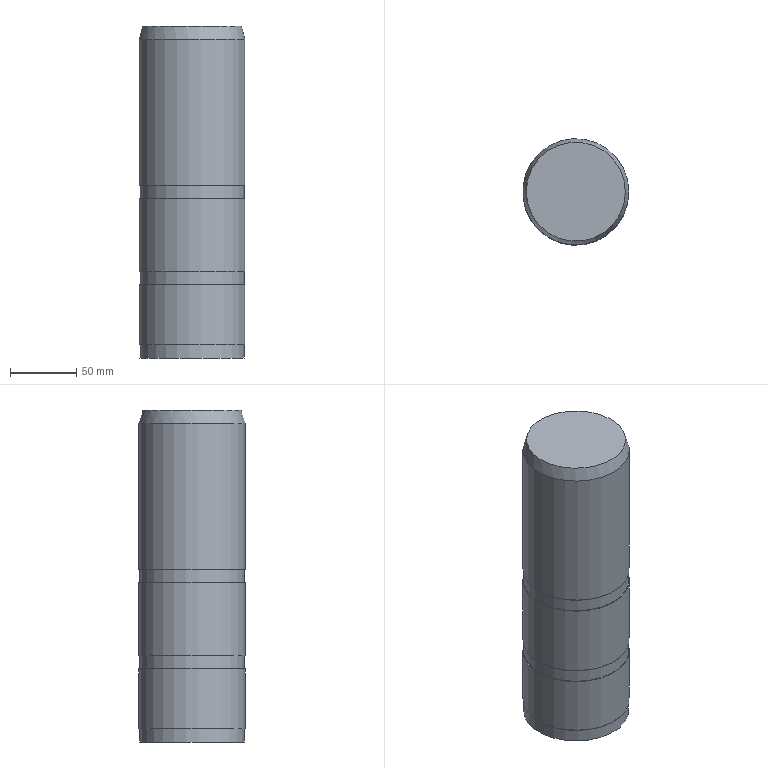Part | NX | features solid 2 | 1 solid | 14 faces | box 80 x 80 x 250 mm | volume 1249599 mm3 | plane 7 | cylinder 6 | cone 1 | commonest cylinder face diameters 79 x3 80 x3
STEP:
#1=CARTESIAN_POINT('',(-910.5,340.,-15.));
#2=VERTEX_POINT('',#1);
#3=CARTESIAN_POINT('',(-950.,340.,-15.));
#4=DIRECTION('',(0.,0.,-1.));
#5=DIRECTION('',(1.,0.,0.));
#6=AXIS2_PLACEMENT_3D('',#3,#4,#5);
#7=CIRCLE('',#6,39.5);
#8=EDGE_CURVE('',#2,#2,#7,.T.);
#9=ORIENTED_EDGE('',*,*,#8,.T.);
#10=EDGE_LOOP('',(#9));
#11=FACE_BOUND('',#10,.T.);
#12=CARTESIAN_POINT('',(-910.5,340.,-25.));
#13=VERTEX_POINT('',#12);
#14=CARTESIAN_POINT('',(-950.,340.,-25.));
#15=DIRECTION('',(0.,0.,-1.));
#16=DIRECTION('',(1.,0.,0.));
#17=AXIS2_PLACEMENT_3D('',#14,#15,#16);
#18=CIRCLE('',#17,39.5);
#19=EDGE_CURVE('',#13,#13,#18,.T.);
#20=ORIENTED_EDGE('',*,*,#19,.F.);
#21=EDGE_LOOP('',(#20));
#22=FACE_BOUND('',#21,.T.);
#23=CARTESIAN_POINT('',(-950.,340.,-15.));
#24=DIRECTION('',(0.,0.,-1.));
#25=DIRECTION('',(-1.,0.,0.));
#26=AXIS2_PLACEMENT_3D('',#23,#24,#25);
#27=CYLINDRICAL_SURFACE('',#26,39.5);
#28=ADVANCED_FACE('',(#11,#22),#27,.T.);
#29=CARTESIAN_POINT('',(-910.,340.,-15.));
#30=VERTEX_POINT('',#29);
#31=CARTESIAN_POINT('',(-950.,340.,-15.));
#32=DIRECTION('',(0.,0.,-1.));
#33=DIRECTION('',(1.,0.,0.));
#34=AXIS2_PLACEMENT_3D('',#31,#32,#33);
#35=CIRCLE('',#34,40.);
#36=EDGE_CURVE('',#30,#30,#35,.T.);
#37=ORIENTED_EDGE('',*,*,#36,.T.);
#38=EDGE_LOOP('',(#37));
#39=FACE_BOUND('',#38,.T.);
#40=ORIENTED_EDGE('',*,*,#8,.F.);
#41=EDGE_LOOP('',(#40));
#42=FACE_BOUND('',#41,.T.);
#43=CARTESIAN_POINT('',(-950.,340.,-15.));
#44=DIRECTION('',(0.,0.,1.));
#45=DIRECTION('',(1.,0.,0.));
#46=AXIS2_PLACEMENT_3D('',#43,#44,#45);
#47=PLANE('',#46);
#48=ADVANCED_FACE('',(#39,#42),#47,.F.);
#49=CARTESIAN_POINT('',(-910.,340.,95.));
#50=VERTEX_POINT('',#49);
#51=CARTESIAN_POINT('',(-950.,340.,95.));
#52=DIRECTION('',(0.,0.,-1.));
#53=DIRECTION('',(1.,0.,0.));
#54=AXIS2_PLACEMENT_3D('',#51,#52,#53);
#55=CIRCLE('',#54,40.);
#56=EDGE_CURVE('',#50,#50,#55,.T.);
#57=ORIENTED_EDGE('',*,*,#56,.T.);
#58=EDGE_LOOP('',(#57));
#59=FACE_BOUND('',#58,.T.);
#60=ORIENTED_EDGE('',*,*,#36,.F.);
#61=EDGE_LOOP('',(#60));
#62=FACE_BOUND('',#61,.T.);
#63=CARTESIAN_POINT('',(-950.,340.,95.));
#64=DIRECTION('',(0.,0.,-1.));
#65=DIRECTION('',(-1.,0.,0.));
#66=AXIS2_PLACEMENT_3D('',#63,#64,#65);
#67=CYLINDRICAL_SURFACE('',#66,40.);
#68=ADVANCED_FACE('',(#59,#62),#67,.T.);
#69=CARTESIAN_POINT('',(-912.679,340.,105.));
#70=VERTEX_POINT('',#69);
#71=CARTESIAN_POINT('',(-950.,340.,105.));
#72=DIRECTION('',(0.,0.,-1.));
#73=DIRECTION('',(1.,0.,0.));
#74=AXIS2_PLACEMENT_3D('',#71,#72,#73);
#75=CIRCLE('',#74,37.321);
#76=EDGE_CURVE('',#70,#70,#75,.T.);
#77=ORIENTED_EDGE('',*,*,#76,.T.);
#78=EDGE_LOOP('',(#77));
#79=FACE_BOUND('',#78,.T.);
#80=ORIENTED_EDGE('',*,*,#56,.F.);
#81=EDGE_LOOP('',(#80));
#82=FACE_BOUND('',#81,.T.);
#83=CARTESIAN_POINT('',(-950.,340.,95.));
#84=DIRECTION('',(0.,0.,-1.));
#85=DIRECTION('',(1.,0.,0.));
#86=AXIS2_PLACEMENT_3D('',#83,#84,#85);
#87=CONICAL_SURFACE('',#86,40.,0.2618);
#88=ADVANCED_FACE('',(#79,#82),#87,.T.);
#89=ORIENTED_EDGE('',*,*,#76,.F.);
#90=EDGE_LOOP('',(#89));
#91=FACE_BOUND('',#90,.T.);
#92=CARTESIAN_POINT('',(-950.,340.,105.));
#93=DIRECTION('',(0.,0.,1.));
#94=DIRECTION('',(1.,0.,0.));
#95=AXIS2_PLACEMENT_3D('',#92,#93,#94);
#96=PLANE('',#95);
#97=ADVANCED_FACE('',(#91),#96,.T.);
#98=CARTESIAN_POINT('',(-910.,340.,-25.));
#99=VERTEX_POINT('',#98);
#100=CARTESIAN_POINT('',(-950.,340.,-25.));
#101=DIRECTION('',(0.,0.,-1.));
#102=DIRECTION('',(1.,0.,0.));
#103=AXIS2_PLACEMENT_3D('',#100,#101,#102);
#104=CIRCLE('',#103,40.);
#105=EDGE_CURVE('',#99,#99,#104,.T.);
#106=ORIENTED_EDGE('',*,*,#105,.F.);
#107=EDGE_LOOP('',(#106));
#108=FACE_BOUND('',#107,.T.);
#109=ORIENTED_EDGE('',*,*,#19,.T.);
#110=EDGE_LOOP('',(#109));
#111=FACE_BOUND('',#110,.T.);
#112=CARTESIAN_POINT('',(-950.,340.,-25.));
#113=DIRECTION('',(0.,0.,1.));
#114=DIRECTION('',(1.,0.,0.));
#115=AXIS2_PLACEMENT_3D('',#112,#113,#114);
#116=PLANE('',#115);
#117=ADVANCED_FACE('',(#108,#111),#116,.T.);
#118=CARTESIAN_POINT('',(-910.,340.,-80.));
#119=VERTEX_POINT('',#118);
#120=CARTESIAN_POINT('',(-950.,340.,-80.));
#121=DIRECTION('',(0.,0.,-1.));
#122=DIRECTION('',(1.,0.,0.));
#123=AXIS2_PLACEMENT_3D('',#120,#121,#122);
#124=CIRCLE('',#123,40.);
#125=EDGE_CURVE('',#119,#119,#124,.T.);
#126=ORIENTED_EDGE('',*,*,#125,.F.);
#127=EDGE_LOOP('',(#126));
#128=FACE_BOUND('',#127,.T.);
#129=ORIENTED_EDGE('',*,*,#105,.T.);
#130=EDGE_LOOP('',(#129));
#131=FACE_BOUND('',#130,.T.);
#132=CARTESIAN_POINT('',(-950.,340.,-80.));
#133=DIRECTION('',(0.,0.,1.));
#134=DIRECTION('',(1.,0.,0.));
#135=AXIS2_PLACEMENT_3D('',#132,#133,#134);
#136=CYLINDRICAL_SURFACE('',#135,40.);
#137=ADVANCED_FACE('',(#128,#131),#136,.T.);
#138=CARTESIAN_POINT('',(-910.5,340.,-80.));
#139=VERTEX_POINT('',#138);
#140=CARTESIAN_POINT('',(-950.,340.,-80.));
#141=DIRECTION('',(0.,0.,-1.));
#142=DIRECTION('',(1.,0.,0.));
#143=AXIS2_PLACEMENT_3D('',#140,#141,#142);
#144=CIRCLE('',#143,39.5);
#145=EDGE_CURVE('',#139,#139,#144,.T.);
#146=ORIENTED_EDGE('',*,*,#145,.F.);
#147=EDGE_LOOP('',(#146));
#148=FACE_BOUND('',#147,.T.);
#149=ORIENTED_EDGE('',*,*,#125,.T.);
#150=EDGE_LOOP('',(#149));
#151=FACE_BOUND('',#150,.T.);
#152=CARTESIAN_POINT('',(-950.,340.,-80.));
#153=DIRECTION('',(0.,0.,1.));
#154=DIRECTION('',(1.,0.,0.));
#155=AXIS2_PLACEMENT_3D('',#152,#153,#154);
#156=PLANE('',#155);
#157=ADVANCED_FACE('',(#148,#151),#156,.F.);
#158=CARTESIAN_POINT('',(-910.5,340.,-90.));
#159=VERTEX_POINT('',#158);
#160=CARTESIAN_POINT('',(-950.,340.,-90.));
#161=DIRECTION('',(0.,0.,-1.));
#162=DIRECTION('',(1.,0.,0.));
#163=AXIS2_PLACEMENT_3D('',#160,#161,#162);
#164=CIRCLE('',#163,39.5);
#165=EDGE_CURVE('',#159,#159,#164,.F.);
#166=ORIENTED_EDGE('',*,*,#165,.T.);
#167=EDGE_LOOP('',(#166));
#168=FACE_BOUND('',#167,.T.);
#169=ORIENTED_EDGE('',*,*,#145,.T.);
#170=EDGE_LOOP('',(#169));
#171=FACE_BOUND('',#170,.T.);
#172=CARTESIAN_POINT('',(-950.,340.,-90.));
#173=DIRECTION('',(0.,0.,1.));
#174=DIRECTION('',(1.,0.,0.));
#175=AXIS2_PLACEMENT_3D('',#172,#173,#174);
#176=CYLINDRICAL_SURFACE('',#175,39.5);
#177=ADVANCED_FACE('',(#168,#171),#176,.T.);
#178=CARTESIAN_POINT('',(-910.,340.,-135.));
#179=VERTEX_POINT('',#178);
#180=CARTESIAN_POINT('',(-950.,340.,-135.));
#181=DIRECTION('',(0.,0.,-1.));
#182=DIRECTION('',(1.,0.,0.));
#183=AXIS2_PLACEMENT_3D('',#180,#181,#182);
#184=CIRCLE('',#183,40.);
#185=EDGE_CURVE('',#179,#179,#184,.T.);
#186=ORIENTED_EDGE('',*,*,#185,.F.);
#187=EDGE_LOOP('',(#186));
#188=FACE_BOUND('',#187,.T.);
#189=CARTESIAN_POINT('',(-910.,340.,-90.));
#190=VERTEX_POINT('',#189);
#191=CARTESIAN_POINT('',(-950.,340.,-90.));
#192=DIRECTION('',(0.,0.,-1.));
#193=DIRECTION('',(1.,0.,0.));
#194=AXIS2_PLACEMENT_3D('',#191,#192,#193);
#195=CIRCLE('',#194,40.);
#196=EDGE_CURVE('',#190,#190,#195,.T.);
#197=ORIENTED_EDGE('',*,*,#196,.T.);
#198=EDGE_LOOP('',(#197));
#199=FACE_BOUND('',#198,.T.);
#200=CARTESIAN_POINT('',(-950.,340.,-135.));
#201=DIRECTION('',(0.,0.,1.));
#202=DIRECTION('',(1.,0.,0.));
#203=AXIS2_PLACEMENT_3D('',#200,#201,#202);
#204=CYLINDRICAL_SURFACE('',#203,40.);
#205=ADVANCED_FACE('',(#188,#199),#204,.T.);
#206=CARTESIAN_POINT('',(-910.5,340.,-135.));
#207=VERTEX_POINT('',#206);
#208=CARTESIAN_POINT('',(-950.,340.,-135.));
#209=DIRECTION('',(0.,0.,-1.));
#210=DIRECTION('',(1.,0.,0.));
#211=AXIS2_PLACEMENT_3D('',#208,#209,#210);
#212=CIRCLE('',#211,39.5);
#213=EDGE_CURVE('',#207,#207,#212,.T.);
#214=ORIENTED_EDGE('',*,*,#213,.F.);
#215=EDGE_LOOP('',(#214));
#216=FACE_BOUND('',#215,.T.);
#217=ORIENTED_EDGE('',*,*,#185,.T.);
#218=EDGE_LOOP('',(#217));
#219=FACE_BOUND('',#218,.T.);
#220=CARTESIAN_POINT('',(-950.,340.,-135.));
#221=DIRECTION('',(0.,0.,1.));
#222=DIRECTION('',(1.,0.,0.));
#223=AXIS2_PLACEMENT_3D('',#220,#221,#222);
#224=PLANE('',#223);
#225=ADVANCED_FACE('',(#216,#219),#224,.F.);
#226=ORIENTED_EDGE('',*,*,#165,.F.);
#227=EDGE_LOOP('',(#226));
#228=FACE_BOUND('',#227,.T.);
#229=ORIENTED_EDGE('',*,*,#196,.F.);
#230=EDGE_LOOP('',(#229));
#231=FACE_BOUND('',#230,.T.);
#232=CARTESIAN_POINT('',(-950.,340.,-90.));
#233=DIRECTION('',(0.,0.,1.));
#234=DIRECTION('',(1.,0.,0.));
#235=AXIS2_PLACEMENT_3D('',#232,#233,#234);
#236=PLANE('',#235);
#237=ADVANCED_FACE('',(#228,#231),#236,.T.);
#238=CARTESIAN_POINT('',(-910.5,340.,-145.));
#239=VERTEX_POINT('',#238);
#240=CARTESIAN_POINT('',(-950.,340.,-145.));
#241=DIRECTION('',(0.,0.,-1.));
#242=DIRECTION('',(1.,0.,0.));
#243=AXIS2_PLACEMENT_3D('',#240,#241,#242);
#244=CIRCLE('',#243,39.5);
#245=EDGE_CURVE('',#239,#239,#244,.T.);
#246=ORIENTED_EDGE('',*,*,#245,.F.);
#247=EDGE_LOOP('',(#246));
#248=FACE_BOUND('',#247,.T.);
#249=ORIENTED_EDGE('',*,*,#213,.T.);
#250=EDGE_LOOP('',(#249));
#251=FACE_BOUND('',#250,.T.);
#252=CARTESIAN_POINT('',(-950.,340.,-145.));
#253=DIRECTION('',(0.,0.,1.));
#254=DIRECTION('',(1.,0.,0.));
#255=AXIS2_PLACEMENT_3D('',#252,#253,#254);
#256=CYLINDRICAL_SURFACE('',#255,39.5);
#257=ADVANCED_FACE('',(#248,#251),#256,.T.);
#258=ORIENTED_EDGE('',*,*,#245,.T.);
#259=EDGE_LOOP('',(#258));
#260=FACE_BOUND('',#259,.T.);
#261=CARTESIAN_POINT('',(-950.,340.,-145.));
#262=DIRECTION('',(0.,0.,1.));
#263=DIRECTION('',(1.,0.,0.));
#264=AXIS2_PLACEMENT_3D('',#261,#262,#263);
#265=PLANE('',#264);
#266=ADVANCED_FACE('',(#260),#265,.F.);
#267=CLOSED_SHELL('',(#28,#48,#68,#88,#97,#117,#137,#157,#177,#205,#225,#237,#257,#266));
#268=MANIFOLD_SOLID_BREP('',#267);
#269=(LENGTH_UNIT()NAMED_UNIT(*)SI_UNIT(.MILLI.,.METRE.));
#270=UNCERTAINTY_MEASURE_WITH_UNIT(LENGTH_MEASURE(0.00001),#269,'','');
#271=(NAMED_UNIT(*)PLANE_ANGLE_UNIT()SI_UNIT($,.RADIAN.));
#272=(NAMED_UNIT(*)SI_UNIT($,.STERADIAN.)SOLID_ANGLE_UNIT());
#273=(GEOMETRIC_REPRESENTATION_CONTEXT(3)GLOBAL_UNCERTAINTY_ASSIGNED_CONTEXT((#270))GLOBAL_UNIT_ASSIGNED_CONTEXT((#269,#271,#272))REPRESENTATION_CONTEXT('',''));
#274=ADVANCED_BREP_SHAPE_REPRESENTATION('',(#268),#273);